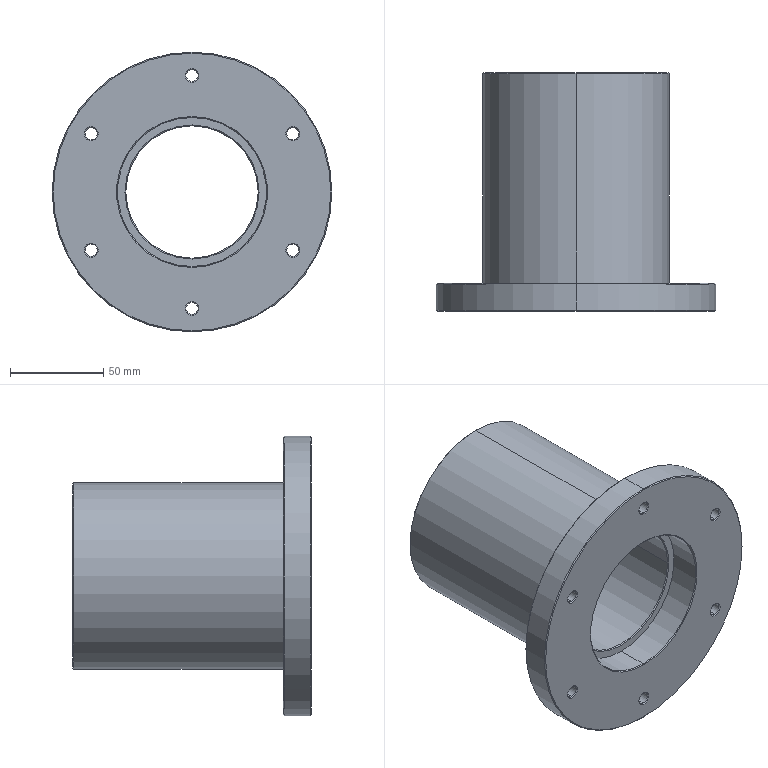Part | STEP file | 05-03 Turntable seat | 1 solid | 95 faces | box 150 x 128 x 150 mm | volume 603065 mm3 | cone 50 | cylinder 34 | plane 11 | commonest cylinder face diameters 6.5 x12 12 x12 80 x4 71 x2 100 x2 150 x2